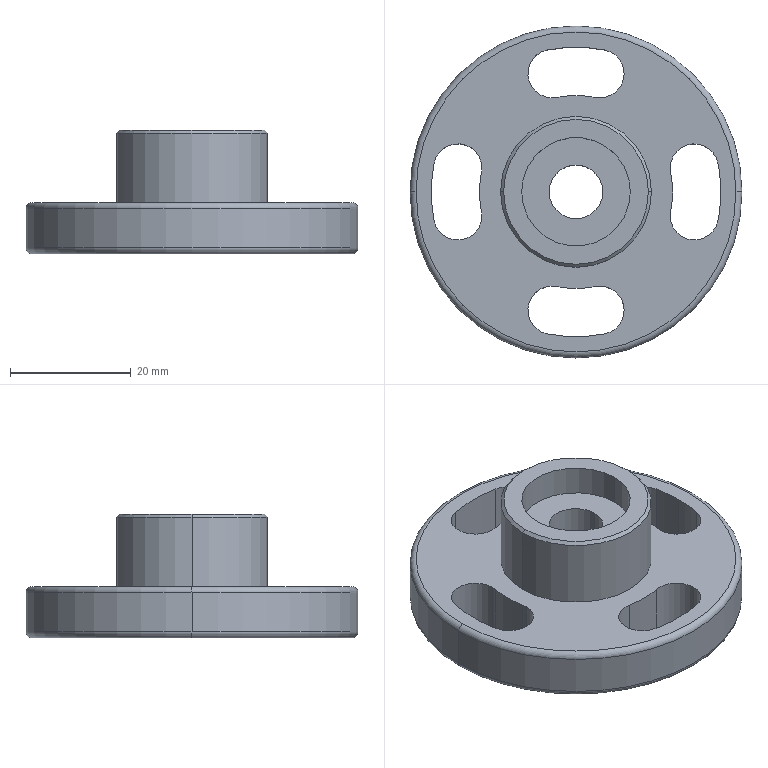Part | SolidWorks | features BaseBody 1 | 1 solid | 43 faces | box 55 x 55 x 20.5 mm | volume 18615 mm3 | cylinder 32 | plane 5 | torus 4 | cone 2 | commonest cylinder face diameters 8 x12 32 x5 48 x5 8.9 x2 15.5 x2 18 x2
STEP:
#1=CARTESIAN_POINT('',(7.973,19.601,0.));
#2=VERTEX_POINT('',#1);
#3=CARTESIAN_POINT('',(4.768,23.522,0.));
#4=VERTEX_POINT('',#3);
#5=CARTESIAN_POINT('',(3.973,19.601,0.));
#6=DIRECTION('',(0.,0.,1.));
#7=DIRECTION('',(1.,0.,0.));
#8=AXIS2_PLACEMENT_3D('',#5,#6,#7);
#9=CIRCLE('',#8,4.);
#10=EDGE_CURVE('',#2,#4,#9,.T.);
#11=ORIENTED_EDGE('',*,*,#10,.F.);
#12=CARTESIAN_POINT('',(7.973,19.601,8.5));
#13=VERTEX_POINT('',#12);
#14=CARTESIAN_POINT('',(7.973,19.601,-1.5));
#15=DIRECTION('',(0.,0.,1.));
#16=VECTOR('',#15,1000.);
#17=LINE('',#14,#16);
#18=EDGE_CURVE('',#2,#13,#17,.T.);
#19=ORIENTED_EDGE('',*,*,#18,.T.);
#20=CARTESIAN_POINT('',(4.768,23.522,8.5));
#21=VERTEX_POINT('',#20);
#22=CARTESIAN_POINT('',(3.973,19.601,8.5));
#23=DIRECTION('',(0.,0.,1.));
#24=DIRECTION('',(1.,0.,0.));
#25=AXIS2_PLACEMENT_3D('',#22,#23,#24);
#26=CIRCLE('',#25,4.);
#27=EDGE_CURVE('',#13,#21,#26,.T.);
#28=ORIENTED_EDGE('',*,*,#27,.T.);
#29=CARTESIAN_POINT('',(4.768,23.522,-1.5));
#30=DIRECTION('',(0.,0.,1.));
#31=VECTOR('',#30,1000.);
#32=LINE('',#29,#31);
#33=EDGE_CURVE('',#4,#21,#32,.T.);
#34=ORIENTED_EDGE('',*,*,#33,.F.);
#35=EDGE_LOOP('',(#11,#19,#28,#34));
#36=FACE_OUTER_BOUND('',#35,.T.);
#37=CARTESIAN_POINT('',(3.973,19.601,-1.5));
#38=DIRECTION('',(0.,0.,1.));
#39=DIRECTION('',(1.,0.,0.));
#40=AXIS2_PLACEMENT_3D('',#37,#38,#39);
#41=CYLINDRICAL_SURFACE('',#40,4.);
#42=ADVANCED_FACE('',(#36),#41,.F.);
#43=CARTESIAN_POINT('',(24.,0.,0.));
#44=VERTEX_POINT('',#43);
#45=CARTESIAN_POINT('',(23.522,4.768,0.));
#46=VERTEX_POINT('',#45);
#47=CARTESIAN_POINT('',(0.,0.,0.));
#48=DIRECTION('',(0.,0.,1.));
#49=DIRECTION('',(1.,0.,0.));
#50=AXIS2_PLACEMENT_3D('',#47,#48,#49);
#51=CIRCLE('',#50,24.);
#52=EDGE_CURVE('',#44,#46,#51,.T.);
#53=ORIENTED_EDGE('',*,*,#52,.F.);
#54=CARTESIAN_POINT('',(24.,0.,8.5));
#55=VERTEX_POINT('',#54);
#56=CARTESIAN_POINT('',(24.,0.,-1.5));
#57=DIRECTION('',(0.,0.,1.));
#58=VECTOR('',#57,1000.);
#59=LINE('',#56,#58);
#60=EDGE_CURVE('',#44,#55,#59,.T.);
#61=ORIENTED_EDGE('',*,*,#60,.T.);
#62=CARTESIAN_POINT('',(23.522,4.768,8.5));
#63=VERTEX_POINT('',#62);
#64=CARTESIAN_POINT('',(0.,0.,8.5));
#65=DIRECTION('',(0.,0.,1.));
#66=DIRECTION('',(1.,0.,0.));
#67=AXIS2_PLACEMENT_3D('',#64,#65,#66);
#68=CIRCLE('',#67,24.);
#69=EDGE_CURVE('',#55,#63,#68,.T.);
#70=ORIENTED_EDGE('',*,*,#69,.T.);
#71=CARTESIAN_POINT('',(23.522,4.768,-1.5));
#72=DIRECTION('',(0.,0.,1.));
#73=VECTOR('',#72,1000.);
#74=LINE('',#71,#73);
#75=EDGE_CURVE('',#46,#63,#74,.T.);
#76=ORIENTED_EDGE('',*,*,#75,.F.);
#77=EDGE_LOOP('',(#53,#61,#70,#76));
#78=FACE_OUTER_BOUND('',#77,.T.);
#79=CARTESIAN_POINT('',(0.,0.,-1.5));
#80=DIRECTION('',(0.,0.,1.));
#81=DIRECTION('',(1.,0.,0.));
#82=AXIS2_PLACEMENT_3D('',#79,#80,#81);
#83=CYLINDRICAL_SURFACE('',#82,24.);
#84=ADVANCED_FACE('',(#78),#83,.F.);
#85=CARTESIAN_POINT('',(16.,0.,0.));
#86=VERTEX_POINT('',#85);
#87=CARTESIAN_POINT('',(15.681,-3.179,0.));
#88=VERTEX_POINT('',#87);
#89=CARTESIAN_POINT('',(0.,0.,0.));
#90=DIRECTION('',(0.,0.,-1.));
#91=DIRECTION('',(1.,0.,0.));
#92=AXIS2_PLACEMENT_3D('',#89,#90,#91);
#93=CIRCLE('',#92,16.);
#94=EDGE_CURVE('',#86,#88,#93,.T.);
#95=ORIENTED_EDGE('',*,*,#94,.F.);
#96=CARTESIAN_POINT('',(16.,0.,8.5));
#97=VERTEX_POINT('',#96);
#98=CARTESIAN_POINT('',(16.,0.,-1.5));
#99=DIRECTION('',(0.,0.,1.));
#100=VECTOR('',#99,1000.);
#101=LINE('',#98,#100);
#102=EDGE_CURVE('',#86,#97,#101,.T.);
#103=ORIENTED_EDGE('',*,*,#102,.T.);
#104=CARTESIAN_POINT('',(15.681,-3.179,8.5));
#105=VERTEX_POINT('',#104);
#106=CARTESIAN_POINT('',(0.,0.,8.5));
#107=DIRECTION('',(0.,0.,-1.));
#108=DIRECTION('',(1.,0.,0.));
#109=AXIS2_PLACEMENT_3D('',#106,#107,#108);
#110=CIRCLE('',#109,16.);
#111=EDGE_CURVE('',#97,#105,#110,.T.);
#112=ORIENTED_EDGE('',*,*,#111,.T.);
#113=CARTESIAN_POINT('',(15.681,-3.179,-1.5));
#114=DIRECTION('',(0.,0.,1.));
#115=VECTOR('',#114,1000.);
#116=LINE('',#113,#115);
#117=EDGE_CURVE('',#88,#105,#116,.T.);
#118=ORIENTED_EDGE('',*,*,#117,.F.);
#119=EDGE_LOOP('',(#95,#103,#112,#118));
#120=FACE_OUTER_BOUND('',#119,.T.);
#121=CARTESIAN_POINT('',(0.,0.,-1.5));
#122=DIRECTION('',(0.,0.,1.));
#123=DIRECTION('',(1.,0.,0.));
#124=AXIS2_PLACEMENT_3D('',#121,#122,#123);
#125=CYLINDRICAL_SURFACE('',#124,16.);
#126=ADVANCED_FACE('',(#120),#125,.T.);
#127=CARTESIAN_POINT('',(7.973,-19.601,0.));
#128=VERTEX_POINT('',#127);
#129=CARTESIAN_POINT('',(3.179,-15.681,0.));
#130=VERTEX_POINT('',#129);
#131=CARTESIAN_POINT('',(3.973,-19.601,0.));
#132=DIRECTION('',(0.,0.,1.));
#133=DIRECTION('',(1.,0.,0.));
#134=AXIS2_PLACEMENT_3D('',#131,#132,#133);
#135=CIRCLE('',#134,4.);
#136=EDGE_CURVE('',#128,#130,#135,.T.);
#137=ORIENTED_EDGE('',*,*,#136,.F.);
#138=CARTESIAN_POINT('',(7.973,-19.601,8.5));
#139=VERTEX_POINT('',#138);
#140=CARTESIAN_POINT('',(7.973,-19.601,-1.5));
#141=DIRECTION('',(0.,0.,1.));
#142=VECTOR('',#141,1000.);
#143=LINE('',#140,#142);
#144=EDGE_CURVE('',#128,#139,#143,.T.);
#145=ORIENTED_EDGE('',*,*,#144,.T.);
#146=CARTESIAN_POINT('',(3.179,-15.681,8.5));
#147=VERTEX_POINT('',#146);
#148=CARTESIAN_POINT('',(3.973,-19.601,8.5));
#149=DIRECTION('',(0.,0.,1.));
#150=DIRECTION('',(1.,0.,0.));
#151=AXIS2_PLACEMENT_3D('',#148,#149,#150);
#152=CIRCLE('',#151,4.);
#153=EDGE_CURVE('',#139,#147,#152,.T.);
#154=ORIENTED_EDGE('',*,*,#153,.T.);
#155=CARTESIAN_POINT('',(3.179,-15.681,-1.5));
#156=DIRECTION('',(0.,0.,1.));
#157=VECTOR('',#156,1000.);
#158=LINE('',#155,#157);
#159=EDGE_CURVE('',#130,#147,#158,.T.);
#160=ORIENTED_EDGE('',*,*,#159,.F.);
#161=EDGE_LOOP('',(#137,#145,#154,#160));
#162=FACE_OUTER_BOUND('',#161,.T.);
#163=CARTESIAN_POINT('',(3.973,-19.601,-1.5));
#164=DIRECTION('',(0.,0.,1.));
#165=DIRECTION('',(1.,0.,0.));
#166=AXIS2_PLACEMENT_3D('',#163,#164,#165);
#167=CYLINDRICAL_SURFACE('',#166,4.);
#168=ADVANCED_FACE('',(#162),#167,.F.);
#169=CARTESIAN_POINT('',(-15.601,-3.973,0.));
#170=VERTEX_POINT('',#169);
#171=CARTESIAN_POINT('',(-15.681,-3.179,0.));
#172=VERTEX_POINT('',#171);
#173=CARTESIAN_POINT('',(-19.601,-3.973,0.));
#174=DIRECTION('',(0.,0.,1.));
#175=DIRECTION('',(1.,0.,0.));
#176=AXIS2_PLACEMENT_3D('',#173,#174,#175);
#177=CIRCLE('',#176,4.);
#178=EDGE_CURVE('',#170,#172,#177,.T.);
#179=ORIENTED_EDGE('',*,*,#178,.F.);
#180=CARTESIAN_POINT('',(-15.601,-3.973,8.5));
#181=VERTEX_POINT('',#180);
#182=CARTESIAN_POINT('',(-15.601,-3.973,-1.5));
#183=DIRECTION('',(0.,0.,1.));
#184=VECTOR('',#183,1000.);
#185=LINE('',#182,#184);
#186=EDGE_CURVE('',#170,#181,#185,.T.);
#187=ORIENTED_EDGE('',*,*,#186,.T.);
#188=CARTESIAN_POINT('',(-15.681,-3.179,8.5));
#189=VERTEX_POINT('',#188);
#190=CARTESIAN_POINT('',(-19.601,-3.973,8.5));
#191=DIRECTION('',(0.,0.,1.));
#192=DIRECTION('',(1.,0.,0.));
#193=AXIS2_PLACEMENT_3D('',#190,#191,#192);
#194=CIRCLE('',#193,4.);
#195=EDGE_CURVE('',#181,#189,#194,.T.);
#196=ORIENTED_EDGE('',*,*,#195,.T.);
#197=CARTESIAN_POINT('',(-15.681,-3.179,-1.5));
#198=DIRECTION('',(0.,0.,1.));
#199=VECTOR('',#198,1000.);
#200=LINE('',#197,#199);
#201=EDGE_CURVE('',#172,#189,#200,.T.);
#202=ORIENTED_EDGE('',*,*,#201,.F.);
#203=EDGE_LOOP('',(#179,#187,#196,#202));
#204=FACE_OUTER_BOUND('',#203,.T.);
#205=CARTESIAN_POINT('',(-19.601,-3.973,-1.5));
#206=DIRECTION('',(0.,0.,1.));
#207=DIRECTION('',(1.,0.,0.));
#208=AXIS2_PLACEMENT_3D('',#205,#206,#207);
#209=CYLINDRICAL_SURFACE('',#208,4.);
#210=ADVANCED_FACE('',(#204),#209,.F.);
#211=CARTESIAN_POINT('',(-15.601,3.973,0.));
#212=VERTEX_POINT('',#211);
#213=CARTESIAN_POINT('',(-23.522,4.768,0.));
#214=VERTEX_POINT('',#213);
#215=CARTESIAN_POINT('',(-19.601,3.973,0.));
#216=DIRECTION('',(0.,0.,1.));
#217=DIRECTION('',(1.,0.,0.));
#218=AXIS2_PLACEMENT_3D('',#215,#216,#217);
#219=CIRCLE('',#218,4.);
#220=EDGE_CURVE('',#212,#214,#219,.T.);
#221=ORIENTED_EDGE('',*,*,#220,.F.);
#222=CARTESIAN_POINT('',(-15.601,3.973,8.5));
#223=VERTEX_POINT('',#222);
#224=CARTESIAN_POINT('',(-15.601,3.973,-1.5));
#225=DIRECTION('',(0.,0.,1.));
#226=VECTOR('',#225,1000.);
#227=LINE('',#224,#226);
#228=EDGE_CURVE('',#212,#223,#227,.T.);
#229=ORIENTED_EDGE('',*,*,#228,.T.);
#230=CARTESIAN_POINT('',(-23.522,4.768,8.5));
#231=VERTEX_POINT('',#230);
#232=CARTESIAN_POINT('',(-19.601,3.973,8.5));
#233=DIRECTION('',(0.,0.,1.));
#234=DIRECTION('',(1.,0.,0.));
#235=AXIS2_PLACEMENT_3D('',#232,#233,#234);
#236=CIRCLE('',#235,4.);
#237=EDGE_CURVE('',#223,#231,#236,.T.);
#238=ORIENTED_EDGE('',*,*,#237,.T.);
#239=CARTESIAN_POINT('',(-23.522,4.768,-1.5));
#240=DIRECTION('',(0.,0.,1.));
#241=VECTOR('',#240,1000.);
#242=LINE('',#239,#241);
#243=EDGE_CURVE('',#214,#231,#242,.T.);
#244=ORIENTED_EDGE('',*,*,#243,.F.);
#245=EDGE_LOOP('',(#221,#229,#238,#244));
#246=FACE_OUTER_BOUND('',#245,.T.);
#247=CARTESIAN_POINT('',(-19.601,3.973,-1.5));
#248=DIRECTION('',(0.,0.,1.));
#249=DIRECTION('',(1.,0.,0.));
#250=AXIS2_PLACEMENT_3D('',#247,#248,#249);
#251=CYLINDRICAL_SURFACE('',#250,4.);
#252=ADVANCED_FACE('',(#246),#251,.F.);
#253=CARTESIAN_POINT('',(-27.5,0.,7.5));
#254=VERTEX_POINT('',#253);
#255=CARTESIAN_POINT('',(27.5,0.,7.5));
#256=VERTEX_POINT('',#255);
#257=CARTESIAN_POINT('',(0.,0.,7.5));
#258=DIRECTION('',(0.,0.,-1.));
#259=DIRECTION('',(1.,0.,0.));
#260=AXIS2_PLACEMENT_3D('',#257,#258,#259);
#261=CIRCLE('',#260,27.5);
#262=EDGE_CURVE('',#254,#256,#261,.T.);
#263=ORIENTED_EDGE('',*,*,#262,.F.);
#264=CARTESIAN_POINT('',(-26.5,0.,8.5));
#265=VERTEX_POINT('',#264);
#266=CARTESIAN_POINT('',(-26.5,0.,7.5));
#267=DIRECTION('',(0.,1.,0.));
#268=DIRECTION('',(-1.,0.,0.));
#269=AXIS2_PLACEMENT_3D('',#266,#267,#268);
#270=CIRCLE('',#269,1.);
#271=EDGE_CURVE('',#254,#265,#270,.T.);
#272=ORIENTED_EDGE('',*,*,#271,.T.);
#273=CARTESIAN_POINT('',(26.5,0.,8.5));
#274=VERTEX_POINT('',#273);
#275=CARTESIAN_POINT('',(0.,0.,8.5));
#276=DIRECTION('',(0.,0.,1.));
#277=DIRECTION('',(1.,0.,0.));
#278=AXIS2_PLACEMENT_3D('',#275,#276,#277);
#279=CIRCLE('',#278,26.5);
#280=EDGE_CURVE('',#274,#265,#279,.T.);
#281=ORIENTED_EDGE('',*,*,#280,.F.);
#282=CARTESIAN_POINT('',(26.5,0.,7.5));
#283=DIRECTION('',(0.,-1.,0.));
#284=DIRECTION('',(0.,0.,-1.));
#285=AXIS2_PLACEMENT_3D('',#282,#283,#284);
#286=CIRCLE('',#285,1.);
#287=EDGE_CURVE('',#256,#274,#286,.T.);
#288=ORIENTED_EDGE('',*,*,#287,.F.);
#289=EDGE_LOOP('',(#263,#272,#281,#288));
#290=FACE_OUTER_BOUND('',#289,.T.);
#291=CARTESIAN_POINT('',(0.,0.,7.5));
#292=DIRECTION('',(0.,0.,1.));
#293=DIRECTION('',(1.,0.,0.));
#294=AXIS2_PLACEMENT_3D('',#291,#292,#293);
#295=TOROIDAL_SURFACE('',#294,26.5,1.);
#296=ADVANCED_FACE('',(#290),#295,.T.);
#297=CARTESIAN_POINT('',(-26.5,0.,0.));
#298=VERTEX_POINT('',#297);
#299=CARTESIAN_POINT('',(26.5,0.,0.));
#300=VERTEX_POINT('',#299);
#301=CARTESIAN_POINT('',(0.,0.,0.));
#302=DIRECTION('',(0.,0.,-1.));
#303=DIRECTION('',(1.,0.,0.));
#304=AXIS2_PLACEMENT_3D('',#301,#302,#303);
#305=CIRCLE('',#304,26.5);
#306=EDGE_CURVE('',#298,#300,#305,.T.);
#307=ORIENTED_EDGE('',*,*,#306,.F.);
#308=CARTESIAN_POINT('',(-27.5,0.,1.));
#309=VERTEX_POINT('',#308);
#310=CARTESIAN_POINT('',(-26.5,0.,1.));
#311=DIRECTION('',(0.,1.,0.));
#312=DIRECTION('',(-1.,0.,0.));
#313=AXIS2_PLACEMENT_3D('',#310,#311,#312);
#314=CIRCLE('',#313,1.);
#315=EDGE_CURVE('',#298,#309,#314,.T.);
#316=ORIENTED_EDGE('',*,*,#315,.T.);
#317=CARTESIAN_POINT('',(27.5,0.,1.));
#318=VERTEX_POINT('',#317);
#319=CARTESIAN_POINT('',(0.,0.,1.));
#320=DIRECTION('',(0.,0.,1.));
#321=DIRECTION('',(1.,0.,0.));
#322=AXIS2_PLACEMENT_3D('',#319,#320,#321);
#323=CIRCLE('',#322,27.5);
#324=EDGE_CURVE('',#318,#309,#323,.T.);
#325=ORIENTED_EDGE('',*,*,#324,.F.);
#326=CARTESIAN_POINT('',(26.5,0.,1.));
#327=DIRECTION('',(0.,-1.,0.));
#328=DIRECTION('',(0.,0.,-1.));
#329=AXIS2_PLACEMENT_3D('',#326,#327,#328);
#330=CIRCLE('',#329,1.);
#331=EDGE_CURVE('',#300,#318,#330,.T.);
#332=ORIENTED_EDGE('',*,*,#331,.F.);
#333=EDGE_LOOP('',(#307,#316,#325,#332));
#334=FACE_OUTER_BOUND('',#333,.T.);
#335=CARTESIAN_POINT('',(0.,0.,1.));
#336=DIRECTION('',(0.,0.,1.));
#337=DIRECTION('',(1.,0.,0.));
#338=AXIS2_PLACEMENT_3D('',#335,#336,#337);
#339=TOROIDAL_SURFACE('',#338,26.5,1.);
#340=ADVANCED_FACE('',(#334),#339,.T.);
#341=CARTESIAN_POINT('',(12.,0.,20.5));
#342=VERTEX_POINT('',#341);
#343=CARTESIAN_POINT('',(-12.,0.,20.5));
#344=VERTEX_POINT('',#343);
#345=CARTESIAN_POINT('',(0.,0.,20.5));
#346=DIRECTION('',(0.,0.,1.));
#347=DIRECTION('',(1.,0.,0.));
#348=AXIS2_PLACEMENT_3D('',#345,#346,#347);
#349=CIRCLE('',#348,12.);
#350=EDGE_CURVE('',#342,#344,#349,.T.);
#351=ORIENTED_EDGE('',*,*,#350,.F.);
#352=CARTESIAN_POINT('',(12.5,0.,20.));
#353=VERTEX_POINT('',#352);
#354=CARTESIAN_POINT('',(12.,0.,20.5));
#355=DIRECTION('',(0.7071,0.,-0.7071));
#356=VECTOR('',#355,1000.);
#357=LINE('',#354,#356);
#358=EDGE_CURVE('',#342,#353,#357,.T.);
#359=ORIENTED_EDGE('',*,*,#358,.T.);
#360=CARTESIAN_POINT('',(-12.5,0.,20.));
#361=VERTEX_POINT('',#360);
#362=CARTESIAN_POINT('',(0.,0.,20.));
#363=DIRECTION('',(0.,0.,-1.));
#364=DIRECTION('',(1.,0.,0.));
#365=AXIS2_PLACEMENT_3D('',#362,#363,#364);
#366=CIRCLE('',#365,12.5);
#367=EDGE_CURVE('',#361,#353,#366,.T.);
#368=ORIENTED_EDGE('',*,*,#367,.F.);
#369=CARTESIAN_POINT('',(-12.,0.,20.5));
#370=DIRECTION('',(-0.7071,0.,-0.7071));
#371=VECTOR('',#370,1000.);
#372=LINE('',#369,#371);
#373=EDGE_CURVE('',#344,#361,#372,.T.);
#374=ORIENTED_EDGE('',*,*,#373,.F.);
#375=EDGE_LOOP('',(#351,#359,#368,#374));
#376=FACE_OUTER_BOUND('',#375,.T.);
#377=CARTESIAN_POINT('',(0.,0.,20.5));
#378=DIRECTION('',(0.,0.,-1.));
#379=DIRECTION('',(-1.,0.,0.));
#380=AXIS2_PLACEMENT_3D('',#377,#378,#379);
#381=CONICAL_SURFACE('',#380,12.,0.7854);
#382=ADVANCED_FACE('',(#376),#381,.T.);
#383=CARTESIAN_POINT('',(-9.,0.,15.5));
#384=VERTEX_POINT('',#383);
#385=CARTESIAN_POINT('',(9.,0.,15.5));
#386=VERTEX_POINT('',#385);
#387=CARTESIAN_POINT('',(0.,0.,15.5));
#388=DIRECTION('',(0.,0.,1.));
#389=DIRECTION('',(1.,0.,0.));
#390=AXIS2_PLACEMENT_3D('',#387,#388,#389);
#391=CIRCLE('',#390,9.);
#392=EDGE_CURVE('',#384,#386,#391,.T.);
#393=ORIENTED_EDGE('',*,*,#392,.F.);
#394=CARTESIAN_POINT('',(-9.,0.,20.5));
#395=VERTEX_POINT('',#394);
#396=CARTESIAN_POINT('',(-9.,0.,15.5));
#397=DIRECTION('',(0.,0.,1.));
#398=VECTOR('',#397,1000.);
#399=LINE('',#396,#398);
#400=EDGE_CURVE('',#384,#395,#399,.T.);
#401=ORIENTED_EDGE('',*,*,#400,.T.);
#402=CARTESIAN_POINT('',(9.,0.,20.5));
#403=VERTEX_POINT('',#402);
#404=CARTESIAN_POINT('',(0.,0.,20.5));
#405=DIRECTION('',(0.,0.,1.));
#406=DIRECTION('',(1.,0.,0.));
#407=AXIS2_PLACEMENT_3D('',#404,#405,#406);
#408=CIRCLE('',#407,9.);
#409=EDGE_CURVE('',#395,#403,#408,.T.);
#410=ORIENTED_EDGE('',*,*,#409,.T.);
#411=CARTESIAN_POINT('',(9.,0.,15.5));
#412=DIRECTION('',(0.,0.,1.));
#413=VECTOR('',#412,1000.);
#414=LINE('',#411,#413);
#415=EDGE_CURVE('',#386,#403,#414,.T.);
#416=ORIENTED_EDGE('',*,*,#415,.F.);
#417=EDGE_LOOP('',(#393,#401,#410,#416));
#418=FACE_OUTER_BOUND('',#417,.T.);
#419=CARTESIAN_POINT('',(0.,0.,15.5));
#420=DIRECTION('',(0.,0.,1.));
#421=DIRECTION('',(1.,0.,0.));
#422=AXIS2_PLACEMENT_3D('',#419,#420,#421);
#423=CYLINDRICAL_SURFACE('',#422,9.);
#424=ADVANCED_FACE('',(#418),#423,.F.);
#425=CARTESIAN_POINT('',(7.75,0.,10.));
#426=VERTEX_POINT('',#425);
#427=CARTESIAN_POINT('',(-7.75,0.,10.));
#428=VERTEX_POINT('',#427);
#429=CARTESIAN_POINT('',(0.,0.,10.));
#430=DIRECTION('',(0.,0.,-1.));
#431=DIRECTION('',(-1.,0.,0.));
#432=AXIS2_PLACEMENT_3D('',#429,#430,#431);
#433=CIRCLE('',#432,7.75);
#434=EDGE_CURVE('',#426,#428,#433,.T.);
#435=ORIENTED_EDGE('',*,*,#434,.F.);
#436=CARTESIAN_POINT('',(7.75,0.,0.));
#437=VERTEX_POINT('',#436);
#438=CARTESIAN_POINT('',(7.75,0.,10.));
#439=DIRECTION('',(0.,0.,-1.));
#440=VECTOR('',#439,1000.);
#441=LINE('',#438,#440);
#442=EDGE_CURVE('',#426,#437,#441,.T.);
#443=ORIENTED_EDGE('',*,*,#442,.T.);
#444=CARTESIAN_POINT('',(-7.75,0.,0.));
#445=VERTEX_POINT('',#444);
#446=CARTESIAN_POINT('',(0.,0.,0.));
#447=DIRECTION('',(0.,0.,-1.));
#448=DIRECTION('',(-1.,0.,0.));
#449=AXIS2_PLACEMENT_3D('',#446,#447,#448);
#450=CIRCLE('',#449,7.75);
#451=EDGE_CURVE('',#437,#445,#450,.T.);
#452=ORIENTED_EDGE('',*,*,#451,.T.);
#453=CARTESIAN_POINT('',(-7.75,0.,10.));
#454=DIRECTION('',(0.,0.,-1.));
#455=VECTOR('',#454,1000.);
#456=LINE('',#453,#455);
#457=EDGE_CURVE('',#428,#445,#456,.T.);
#458=ORIENTED_EDGE('',*,*,#457,.F.);
#459=EDGE_LOOP('',(#435,#443,#452,#458));
#460=FACE_OUTER_BOUND('',#459,.T.);
#461=CARTESIAN_POINT('',(0.,0.,10.));
#462=DIRECTION('',(0.,0.,-1.));
#463=DIRECTION('',(-1.,0.,0.));
#464=AXIS2_PLACEMENT_3D('',#461,#462,#463);
#465=CYLINDRICAL_SURFACE('',#464,7.75);
#466=ADVANCED_FACE('',(#460),#465,.F.);
#467=ORIENTED_EDGE('',*,*,#367,.T.);
#468=CARTESIAN_POINT('',(12.5,0.,8.5));
#469=VERTEX_POINT('',#468);
#470=CARTESIAN_POINT('',(12.5,0.,20.5));
#471=DIRECTION('',(0.,0.,-1.));
#472=VECTOR('',#471,1000.);
#473=LINE('',#470,#472);
#474=EDGE_CURVE('',#353,#469,#473,.T.);
#475=ORIENTED_EDGE('',*,*,#474,.T.);
#476=CARTESIAN_POINT('',(-12.5,0.,8.5));
#477=VERTEX_POINT('',#476);
#478=CARTESIAN_POINT('',(0.,0.,8.5));
#479=DIRECTION('',(0.,0.,1.));
#480=DIRECTION('',(1.,0.,0.));
#481=AXIS2_PLACEMENT_3D('',#478,#479,#480);
#482=CIRCLE('',#481,12.5);
#483=EDGE_CURVE('',#469,#477,#482,.T.);
#484=ORIENTED_EDGE('',*,*,#483,.T.);
#485=CARTESIAN_POINT('',(-12.5,0.,20.5));
#486=DIRECTION('',(0.,0.,-1.));
#487=VECTOR('',#486,1000.);
#488=LINE('',#485,#487);
#489=EDGE_CURVE('',#361,#477,#488,.T.);
#490=ORIENTED_EDGE('',*,*,#489,.F.);
#491=EDGE_LOOP('',(#467,#475,#484,#490));
#492=FACE_OUTER_BOUND('',#491,.T.);
#493=CARTESIAN_POINT('',(0.,0.,20.5));
#494=DIRECTION('',(0.,0.,-1.));
#495=DIRECTION('',(-1.,0.,0.));
#496=AXIS2_PLACEMENT_3D('',#493,#494,#495);
#497=CYLINDRICAL_SURFACE('',#496,12.5);
#498=ADVANCED_FACE('',(#492),#497,.T.);
#499=ORIENTED_EDGE('',*,*,#262,.T.);
#500=CARTESIAN_POINT('',(27.5,0.,8.5));
#501=DIRECTION('',(0.,0.,-1.));
#502=VECTOR('',#501,1000.);
#503=LINE('',#500,#502);
#504=EDGE_CURVE('',#256,#318,#503,.T.);
#505=ORIENTED_EDGE('',*,*,#504,.T.);
#506=ORIENTED_EDGE('',*,*,#324,.T.);
#507=CARTESIAN_POINT('',(-27.5,0.,8.5));
#508=DIRECTION('',(0.,0.,-1.));
#509=VECTOR('',#508,1000.);
#510=LINE('',#507,#509);
#511=EDGE_CURVE('',#254,#309,#510,.T.);
#512=ORIENTED_EDGE('',*,*,#511,.F.);
#513=EDGE_LOOP('',(#499,#505,#506,#512));
#514=FACE_OUTER_BOUND('',#513,.T.);
#515=CARTESIAN_POINT('',(0.,0.,8.5));
#516=DIRECTION('',(0.,0.,-1.));
#517=DIRECTION('',(-1.,0.,0.));
#518=AXIS2_PLACEMENT_3D('',#515,#516,#517);
#519=CYLINDRICAL_SURFACE('',#518,27.5);
#520=ADVANCED_FACE('',(#514),#519,.T.);
#521=CARTESIAN_POINT('',(-4.45,0.,15.5));
#522=VERTEX_POINT('',#521);
#523=CARTESIAN_POINT('',(4.45,0.,15.5));
#524=VERTEX_POINT('',#523);
#525=CARTESIAN_POINT('',(0.,0.,15.5));
#526=DIRECTION('',(0.,0.,1.));
#527=DIRECTION('',(1.,0.,0.));
#528=AXIS2_PLACEMENT_3D('',#525,#526,#527);
#529=CIRCLE('',#528,4.45);
#530=EDGE_CURVE('',#522,#524,#529,.T.);
#531=ORIENTED_EDGE('',*,*,#530,.T.);
#532=CARTESIAN_POINT('',(4.45,0.,10.));
#533=VERTEX_POINT('',#532);
#534=CARTESIAN_POINT('',(4.45,0.,8.5));
#535=DIRECTION('',(0.,0.,-1.));
#536=VECTOR('',#535,1000.);
#537=LINE('',#534,#536);
#538=EDGE_CURVE('',#524,#533,#537,.T.);
#539=ORIENTED_EDGE('',*,*,#538,.T.);
#540=CARTESIAN_POINT('',(-4.45,0.,10.));
#541=VERTEX_POINT('',#540);
#542=CARTESIAN_POINT('',(0.,0.,10.));
#543=DIRECTION('',(0.,0.,-1.));
#544=DIRECTION('',(-1.,0.,0.));
#545=AXIS2_PLACEMENT_3D('',#542,#543,#544);
#546=CIRCLE('',#545,4.45);
#547=EDGE_CURVE('',#533,#541,#546,.T.);
#548=ORIENTED_EDGE('',*,*,#547,.T.);
#549=CARTESIAN_POINT('',(-4.45,0.,8.5));
#550=DIRECTION('',(0.,0.,-1.));
#551=VECTOR('',#550,1000.);
#552=LINE('',#549,#551);
#553=EDGE_CURVE('',#522,#541,#552,.T.);
#554=ORIENTED_EDGE('',*,*,#553,.F.);
#555=EDGE_LOOP('',(#531,#539,#548,#554));
#556=FACE_OUTER_BOUND('',#555,.T.);
#557=CARTESIAN_POINT('',(0.,0.,8.5));
#558=DIRECTION('',(0.,0.,-1.));
#559=DIRECTION('',(-1.,0.,0.));
#560=AXIS2_PLACEMENT_3D('',#557,#558,#559);
#561=CYLINDRICAL_SURFACE('',#560,4.45);
#562=ADVANCED_FACE('',(#556),#561,.F.);
#563=ORIENTED_EDGE('',*,*,#538,.F.);
#564=CARTESIAN_POINT('',(0.,0.,15.5));
#565=DIRECTION('',(0.,0.,1.));
#566=DIRECTION('',(1.,0.,0.));
#567=AXIS2_PLACEMENT_3D('',#564,#565,#566);
#568=CIRCLE('',#567,4.45);
#569=EDGE_CURVE('',#524,#522,#568,.T.);
#570=ORIENTED_EDGE('',*,*,#569,.T.);
#571=ORIENTED_EDGE('',*,*,#553,.T.);
#572=CARTESIAN_POINT('',(0.,0.,10.));
#573=DIRECTION('',(0.,0.,-1.));
#574=DIRECTION('',(-1.,0.,0.));
#575=AXIS2_PLACEMENT_3D('',#572,#573,#574);
#576=CIRCLE('',#575,4.45);
#577=EDGE_CURVE('',#541,#533,#576,.T.);
#578=ORIENTED_EDGE('',*,*,#577,.T.);
#579=EDGE_LOOP('',(#563,#570,#571,#578));
#580=FACE_OUTER_BOUND('',#579,.T.);
#581=CARTESIAN_POINT('',(0.,0.,8.5));
#582=DIRECTION('',(0.,0.,-1.));
#583=DIRECTION('',(-1.,0.,0.));
#584=AXIS2_PLACEMENT_3D('',#581,#582,#583);
#585=CYLINDRICAL_SURFACE('',#584,4.45);
#586=ADVANCED_FACE('',(#580),#585,.F.);
#587=CARTESIAN_POINT('',(3.179,15.681,8.5));
#588=VERTEX_POINT('',#587);
#589=CARTESIAN_POINT('',(3.973,19.601,8.5));
#590=DIRECTION('',(0.,0.,1.));
#591=DIRECTION('',(1.,0.,0.));
#592=AXIS2_PLACEMENT_3D('',#589,#590,#591);
#593=CIRCLE('',#592,4.);
#594=EDGE_CURVE('',#588,#13,#593,.T.);
#595=ORIENTED_EDGE('',*,*,#594,.F.);
#596=CARTESIAN_POINT('',(-3.179,15.681,8.5));
#597=VERTEX_POINT('',#596);
#598=CARTESIAN_POINT('',(0.,0.,8.5));
#599=DIRECTION('',(0.,0.,-1.));
#600=DIRECTION('',(1.,0.,0.));
#601=AXIS2_PLACEMENT_3D('',#598,#599,#600);
#602=CIRCLE('',#601,16.);
#603=EDGE_CURVE('',#597,#588,#602,.T.);
#604=ORIENTED_EDGE('',*,*,#603,.F.);
#605=CARTESIAN_POINT('',(-4.768,23.522,8.5));
#606=VERTEX_POINT('',#605);
#607=CARTESIAN_POINT('',(-3.973,19.601,8.5));
#608=DIRECTION('',(0.,0.,1.));
#609=DIRECTION('',(1.,0.,0.));
#610=AXIS2_PLACEMENT_3D('',#607,#608,#609);
#611=CIRCLE('',#610,4.);
#612=EDGE_CURVE('',#606,#597,#611,.T.);
#613=ORIENTED_EDGE('',*,*,#612,.F.);
#614=CARTESIAN_POINT('',(0.,0.,8.5));
#615=DIRECTION('',(0.,0.,1.));
#616=DIRECTION('',(1.,0.,0.));
#617=AXIS2_PLACEMENT_3D('',#614,#615,#616);
#618=CIRCLE('',#617,24.);
#619=EDGE_CURVE('',#21,#606,#618,.T.);
#620=ORIENTED_EDGE('',*,*,#619,.F.);
#621=ORIENTED_EDGE('',*,*,#27,.F.);
#622=EDGE_LOOP('',(#595,#604,#613,#620,#621));
#623=FACE_BOUND('',#622,.T.);
#624=CARTESIAN_POINT('',(23.522,-4.768,8.5));
#625=VERTEX_POINT('',#624);
#626=CARTESIAN_POINT('',(19.601,-3.973,8.5));
#627=DIRECTION('',(0.,0.,1.));
#628=DIRECTION('',(1.,0.,0.));
#629=AXIS2_PLACEMENT_3D('',#626,#627,#628);
#630=CIRCLE('',#629,4.);
#631=EDGE_CURVE('',#105,#625,#630,.T.);
#632=ORIENTED_EDGE('',*,*,#631,.F.);
#633=ORIENTED_EDGE('',*,*,#111,.F.);
#634=CARTESIAN_POINT('',(15.681,3.179,8.5));
#635=VERTEX_POINT('',#634);
#636=CARTESIAN_POINT('',(0.,0.,8.5));
#637=DIRECTION('',(0.,0.,-1.));
#638=DIRECTION('',(1.,0.,0.));
#639=AXIS2_PLACEMENT_3D('',#636,#637,#638);
#640=CIRCLE('',#639,16.);
#641=EDGE_CURVE('',#635,#97,#640,.T.);
#642=ORIENTED_EDGE('',*,*,#641,.F.);
#643=CARTESIAN_POINT('',(19.601,3.973,8.5));
#644=DIRECTION('',(0.,0.,1.));
#645=DIRECTION('',(1.,0.,0.));
#646=AXIS2_PLACEMENT_3D('',#643,#644,#645);
#647=CIRCLE('',#646,4.);
#648=EDGE_CURVE('',#63,#635,#647,.T.);
#649=ORIENTED_EDGE('',*,*,#648,.F.);
#650=ORIENTED_EDGE('',*,*,#69,.F.);
#651=CARTESIAN_POINT('',(0.,0.,8.5));
#652=DIRECTION('',(0.,0.,1.));
#653=DIRECTION('',(1.,0.,0.));
#654=AXIS2_PLACEMENT_3D('',#651,#652,#653);
#655=CIRCLE('',#654,24.);
#656=EDGE_CURVE('',#625,#55,#655,.T.);
#657=ORIENTED_EDGE('',*,*,#656,.F.);
#658=EDGE_LOOP('',(#632,#633,#642,#649,#650,#657));
#659=FACE_BOUND('',#658,.T.);
#660=CARTESIAN_POINT('',(-3.179,-15.681,8.5));
#661=VERTEX_POINT('',#660);
#662=CARTESIAN_POINT('',(-4.768,-23.522,8.5));
#663=VERTEX_POINT('',#662);
#664=CARTESIAN_POINT('',(-3.973,-19.601,8.5));
#665=DIRECTION('',(0.,0.,1.));
#666=DIRECTION('',(1.,0.,0.));
#667=AXIS2_PLACEMENT_3D('',#664,#665,#666);
#668=CIRCLE('',#667,4.);
#669=EDGE_CURVE('',#661,#663,#668,.T.);
#670=ORIENTED_EDGE('',*,*,#669,.F.);
#671=CARTESIAN_POINT('',(0.,0.,8.5));
#672=DIRECTION('',(0.,0.,-1.));
#673=DIRECTION('',(1.,0.,0.));
#674=AXIS2_PLACEMENT_3D('',#671,#672,#673);
#675=CIRCLE('',#674,16.);
#676=EDGE_CURVE('',#147,#661,#675,.T.);
#677=ORIENTED_EDGE('',*,*,#676,.F.);
#678=ORIENTED_EDGE('',*,*,#153,.F.);
#679=CARTESIAN_POINT('',(4.768,-23.522,8.5));
#680=VERTEX_POINT('',#679);
#681=CARTESIAN_POINT('',(3.973,-19.601,8.5));
#682=DIRECTION('',(0.,0.,1.));
#683=DIRECTION('',(1.,0.,0.));
#684=AXIS2_PLACEMENT_3D('',#681,#682,#683);
#685=CIRCLE('',#684,4.);
#686=EDGE_CURVE('',#680,#139,#685,.T.);
#687=ORIENTED_EDGE('',*,*,#686,.F.);
#688=CARTESIAN_POINT('',(0.,0.,8.5));
#689=DIRECTION('',(0.,0.,1.));
#690=DIRECTION('',(1.,0.,0.));
#691=AXIS2_PLACEMENT_3D('',#688,#689,#690);
#692=CIRCLE('',#691,24.);
#693=EDGE_CURVE('',#663,#680,#692,.T.);
#694=ORIENTED_EDGE('',*,*,#693,.F.);
#695=EDGE_LOOP('',(#670,#677,#678,#687,#694));
#696=FACE_BOUND('',#695,.T.);
#697=CARTESIAN_POINT('',(-15.681,3.179,8.5));
#698=VERTEX_POINT('',#697);
#699=CARTESIAN_POINT('',(-19.601,3.973,8.5));
#700=DIRECTION('',(0.,0.,1.));
#701=DIRECTION('',(1.,0.,0.));
#702=AXIS2_PLACEMENT_3D('',#699,#700,#701);
#703=CIRCLE('',#702,4.);
#704=EDGE_CURVE('',#698,#223,#703,.T.);
#705=ORIENTED_EDGE('',*,*,#704,.F.);
#706=CARTESIAN_POINT('',(0.,0.,8.5));
#707=DIRECTION('',(0.,0.,-1.));
#708=DIRECTION('',(1.,0.,0.));
#709=AXIS2_PLACEMENT_3D('',#706,#707,#708);
#710=CIRCLE('',#709,16.);
#711=EDGE_CURVE('',#189,#698,#710,.T.);
#712=ORIENTED_EDGE('',*,*,#711,.F.);
#713=ORIENTED_EDGE('',*,*,#195,.F.);
#714=CARTESIAN_POINT('',(-23.522,-4.768,8.5));
#715=VERTEX_POINT('',#714);
#716=CARTESIAN_POINT('',(-19.601,-3.973,8.5));
#717=DIRECTION('',(0.,0.,1.));
#718=DIRECTION('',(1.,0.,0.));
#719=AXIS2_PLACEMENT_3D('',#716,#717,#718);
#720=CIRCLE('',#719,4.);
#721=EDGE_CURVE('',#715,#181,#720,.T.);
#722=ORIENTED_EDGE('',*,*,#721,.F.);
#723=CARTESIAN_POINT('',(0.,0.,8.5));
#724=DIRECTION('',(0.,0.,1.));
#725=DIRECTION('',(1.,0.,0.));
#726=AXIS2_PLACEMENT_3D('',#723,#724,#725);
#727=CIRCLE('',#726,24.);
#728=EDGE_CURVE('',#231,#715,#727,.T.);
#729=ORIENTED_EDGE('',*,*,#728,.F.);
#730=ORIENTED_EDGE('',*,*,#237,.F.);
#731=EDGE_LOOP('',(#705,#712,#713,#722,#729,#730));
#732=FACE_BOUND('',#731,.T.);
#733=ORIENTED_EDGE('',*,*,#280,.T.);
#734=CARTESIAN_POINT('',(0.,0.,8.5));
#735=DIRECTION('',(0.,0.,1.));
#736=DIRECTION('',(1.,0.,0.));
#737=AXIS2_PLACEMENT_3D('',#734,#735,#736);
#738=CIRCLE('',#737,26.5);
#739=EDGE_CURVE('',#265,#274,#738,.T.);
#740=ORIENTED_EDGE('',*,*,#739,.T.);
#741=EDGE_LOOP('',(#733,#740));
#742=FACE_OUTER_BOUND('',#741,.T.);
#743=CARTESIAN_POINT('',(0.,0.,8.5));
#744=DIRECTION('',(0.,0.,1.));
#745=DIRECTION('',(1.,0.,0.));
#746=AXIS2_PLACEMENT_3D('',#743,#744,#745);
#747=CIRCLE('',#746,12.5);
#748=EDGE_CURVE('',#477,#469,#747,.T.);
#749=ORIENTED_EDGE('',*,*,#748,.F.);
#750=ORIENTED_EDGE('',*,*,#483,.F.);
#751=EDGE_LOOP('',(#749,#750));
#752=FACE_BOUND('',#751,.T.);
#753=CARTESIAN_POINT('',(0.,0.,8.5));
#754=DIRECTION('',(0.,0.,1.));
#755=DIRECTION('',(1.,0.,0.));
#756=AXIS2_PLACEMENT_3D('',#753,#754,#755);
#757=PLANE('',#756);
#758=ADVANCED_FACE('',(#623,#659,#696,#732,#742,#752),#757,.T.);
#759=CARTESIAN_POINT('',(-3.179,15.681,0.));
#760=VERTEX_POINT('',#759);
#761=CARTESIAN_POINT('',(3.179,15.681,0.));
#762=VERTEX_POINT('',#761);
#763=CARTESIAN_POINT('',(0.,0.,0.));
#764=DIRECTION('',(0.,0.,-1.));
#765=DIRECTION('',(1.,0.,0.));
#766=AXIS2_PLACEMENT_3D('',#763,#764,#765);
#767=CIRCLE('',#766,16.);
#768=EDGE_CURVE('',#760,#762,#767,.T.);
#769=ORIENTED_EDGE('',*,*,#768,.T.);
#770=CARTESIAN_POINT('',(3.973,19.601,0.));
#771=DIRECTION('',(0.,0.,1.));
#772=DIRECTION('',(1.,0.,0.));
#773=AXIS2_PLACEMENT_3D('',#770,#771,#772);
#774=CIRCLE('',#773,4.);
#775=EDGE_CURVE('',#762,#2,#774,.T.);
#776=ORIENTED_EDGE('',*,*,#775,.T.);
#777=ORIENTED_EDGE('',*,*,#10,.T.);
#778=CARTESIAN_POINT('',(-4.768,23.522,0.));
#779=VERTEX_POINT('',#778);
#780=CARTESIAN_POINT('',(0.,0.,0.));
#781=DIRECTION('',(0.,0.,1.));
#782=DIRECTION('',(1.,0.,0.));
#783=AXIS2_PLACEMENT_3D('',#780,#781,#782);
#784=CIRCLE('',#783,24.);
#785=EDGE_CURVE('',#4,#779,#784,.T.);
#786=ORIENTED_EDGE('',*,*,#785,.T.);
#787=CARTESIAN_POINT('',(-3.973,19.601,0.));
#788=DIRECTION('',(0.,0.,1.));
#789=DIRECTION('',(1.,0.,0.));
#790=AXIS2_PLACEMENT_3D('',#787,#788,#789);
#791=CIRCLE('',#790,4.);
#792=EDGE_CURVE('',#779,#760,#791,.T.);
#793=ORIENTED_EDGE('',*,*,#792,.T.);
#794=EDGE_LOOP('',(#769,#776,#777,#786,#793));
#795=FACE_BOUND('',#794,.T.);
#796=CARTESIAN_POINT('',(15.681,3.179,0.));
#797=VERTEX_POINT('',#796);
#798=CARTESIAN_POINT('',(0.,0.,0.));
#799=DIRECTION('',(0.,0.,-1.));
#800=DIRECTION('',(1.,0.,0.));
#801=AXIS2_PLACEMENT_3D('',#798,#799,#800);
#802=CIRCLE('',#801,16.);
#803=EDGE_CURVE('',#797,#86,#802,.T.);
#804=ORIENTED_EDGE('',*,*,#803,.T.);
#805=ORIENTED_EDGE('',*,*,#94,.T.);
#806=CARTESIAN_POINT('',(23.522,-4.768,0.));
#807=VERTEX_POINT('',#806);
#808=CARTESIAN_POINT('',(19.601,-3.973,0.));
#809=DIRECTION('',(0.,0.,1.));
#810=DIRECTION('',(1.,0.,0.));
#811=AXIS2_PLACEMENT_3D('',#808,#809,#810);
#812=CIRCLE('',#811,4.);
#813=EDGE_CURVE('',#88,#807,#812,.T.);
#814=ORIENTED_EDGE('',*,*,#813,.T.);
#815=CARTESIAN_POINT('',(0.,0.,0.));
#816=DIRECTION('',(0.,0.,1.));
#817=DIRECTION('',(1.,0.,0.));
#818=AXIS2_PLACEMENT_3D('',#815,#816,#817);
#819=CIRCLE('',#818,24.);
#820=EDGE_CURVE('',#807,#44,#819,.T.);
#821=ORIENTED_EDGE('',*,*,#820,.T.);
#822=ORIENTED_EDGE('',*,*,#52,.T.);
#823=CARTESIAN_POINT('',(19.601,3.973,0.));
#824=DIRECTION('',(0.,0.,1.));
#825=DIRECTION('',(1.,0.,0.));
#826=AXIS2_PLACEMENT_3D('',#823,#824,#825);
#827=CIRCLE('',#826,4.);
#828=EDGE_CURVE('',#46,#797,#827,.T.);
#829=ORIENTED_EDGE('',*,*,#828,.T.);
#830=EDGE_LOOP('',(#804,#805,#814,#821,#822,#829));
#831=FACE_BOUND('',#830,.T.);
#832=CARTESIAN_POINT('',(-3.179,-15.681,0.));
#833=VERTEX_POINT('',#832);
#834=CARTESIAN_POINT('',(0.,0.,0.));
#835=DIRECTION('',(0.,0.,-1.));
#836=DIRECTION('',(1.,0.,0.));
#837=AXIS2_PLACEMENT_3D('',#834,#835,#836);
#838=CIRCLE('',#837,16.);
#839=EDGE_CURVE('',#130,#833,#838,.T.);
#840=ORIENTED_EDGE('',*,*,#839,.T.);
#841=CARTESIAN_POINT('',(-4.768,-23.522,0.));
#842=VERTEX_POINT('',#841);
#843=CARTESIAN_POINT('',(-3.973,-19.601,0.));
#844=DIRECTION('',(0.,0.,1.));
#845=DIRECTION('',(1.,0.,0.));
#846=AXIS2_PLACEMENT_3D('',#843,#844,#845);
#847=CIRCLE('',#846,4.);
#848=EDGE_CURVE('',#833,#842,#847,.T.);
#849=ORIENTED_EDGE('',*,*,#848,.T.);
#850=CARTESIAN_POINT('',(4.768,-23.522,0.));
#851=VERTEX_POINT('',#850);
#852=CARTESIAN_POINT('',(0.,0.,0.));
#853=DIRECTION('',(0.,0.,1.));
#854=DIRECTION('',(1.,0.,0.));
#855=AXIS2_PLACEMENT_3D('',#852,#853,#854);
#856=CIRCLE('',#855,24.);
#857=EDGE_CURVE('',#842,#851,#856,.T.);
#858=ORIENTED_EDGE('',*,*,#857,.T.);
#859=CARTESIAN_POINT('',(3.973,-19.601,0.));
#860=DIRECTION('',(0.,0.,1.));
#861=DIRECTION('',(1.,0.,0.));
#862=AXIS2_PLACEMENT_3D('',#859,#860,#861);
#863=CIRCLE('',#862,4.);
#864=EDGE_CURVE('',#851,#128,#863,.T.);
#865=ORIENTED_EDGE('',*,*,#864,.T.);
#866=ORIENTED_EDGE('',*,*,#136,.T.);
#867=EDGE_LOOP('',(#840,#849,#858,#865,#866));
#868=FACE_BOUND('',#867,.T.);
#869=CARTESIAN_POINT('',(-15.681,3.179,0.));
#870=VERTEX_POINT('',#869);
#871=CARTESIAN_POINT('',(0.,0.,0.));
#872=DIRECTION('',(0.,0.,-1.));
#873=DIRECTION('',(1.,0.,0.));
#874=AXIS2_PLACEMENT_3D('',#871,#872,#873);
#875=CIRCLE('',#874,16.);
#876=EDGE_CURVE('',#172,#870,#875,.T.);
#877=ORIENTED_EDGE('',*,*,#876,.T.);
#878=CARTESIAN_POINT('',(-19.601,3.973,0.));
#879=DIRECTION('',(0.,0.,1.));
#880=DIRECTION('',(1.,0.,0.));
#881=AXIS2_PLACEMENT_3D('',#878,#879,#880);
#882=CIRCLE('',#881,4.);
#883=EDGE_CURVE('',#870,#212,#882,.T.);
#884=ORIENTED_EDGE('',*,*,#883,.T.);
#885=ORIENTED_EDGE('',*,*,#220,.T.);
#886=CARTESIAN_POINT('',(-23.522,-4.768,0.));
#887=VERTEX_POINT('',#886);
#888=CARTESIAN_POINT('',(0.,0.,0.));
#889=DIRECTION('',(0.,0.,1.));
#890=DIRECTION('',(1.,0.,0.));
#891=AXIS2_PLACEMENT_3D('',#888,#889,#890);
#892=CIRCLE('',#891,24.);
#893=EDGE_CURVE('',#214,#887,#892,.T.);
#894=ORIENTED_EDGE('',*,*,#893,.T.);
#895=CARTESIAN_POINT('',(-19.601,-3.973,0.));
#896=DIRECTION('',(0.,0.,1.));
#897=DIRECTION('',(1.,0.,0.));
#898=AXIS2_PLACEMENT_3D('',#895,#896,#897);
#899=CIRCLE('',#898,4.);
#900=EDGE_CURVE('',#887,#170,#899,.T.);
#901=ORIENTED_EDGE('',*,*,#900,.T.);
#902=ORIENTED_EDGE('',*,*,#178,.T.);
#903=EDGE_LOOP('',(#877,#884,#885,#894,#901,#902));
#904=FACE_BOUND('',#903,.T.);
#905=CARTESIAN_POINT('',(0.,0.,0.));
#906=DIRECTION('',(0.,0.,-1.));
#907=DIRECTION('',(1.,0.,0.));
#908=AXIS2_PLACEMENT_3D('',#905,#906,#907);
#909=CIRCLE('',#908,26.5);
#910=EDGE_CURVE('',#300,#298,#909,.T.);
#911=ORIENTED_EDGE('',*,*,#910,.T.);
#912=ORIENTED_EDGE('',*,*,#306,.T.);
#913=EDGE_LOOP('',(#911,#912));
#914=FACE_OUTER_BOUND('',#913,.T.);
#915=CARTESIAN_POINT('',(0.,0.,0.));
#916=DIRECTION('',(0.,0.,-1.));
#917=DIRECTION('',(-1.,0.,0.));
#918=AXIS2_PLACEMENT_3D('',#915,#916,#917);
#919=CIRCLE('',#918,7.75);
#920=EDGE_CURVE('',#445,#437,#919,.T.);
#921=ORIENTED_EDGE('',*,*,#920,.F.);
#922=ORIENTED_EDGE('',*,*,#451,.F.);
#923=EDGE_LOOP('',(#921,#922));
#924=FACE_BOUND('',#923,.T.);
#925=CARTESIAN_POINT('',(0.,0.,0.));
#926=DIRECTION('',(0.,0.,1.));
#927=DIRECTION('',(1.,0.,0.));
#928=AXIS2_PLACEMENT_3D('',#925,#926,#927);
#929=PLANE('',#928);
#930=ADVANCED_FACE('',(#795,#831,#868,#904,#914,#924),#929,.F.);
#931=ORIENTED_EDGE('',*,*,#504,.F.);
#932=CARTESIAN_POINT('',(0.,0.,7.5));
#933=DIRECTION('',(0.,0.,-1.));
#934=DIRECTION('',(1.,0.,0.));
#935=AXIS2_PLACEMENT_3D('',#932,#933,#934);
#936=CIRCLE('',#935,27.5);
#937=EDGE_CURVE('',#256,#254,#936,.T.);
#938=ORIENTED_EDGE('',*,*,#937,.T.);
#939=ORIENTED_EDGE('',*,*,#511,.T.);
#940=CARTESIAN_POINT('',(0.,0.,1.));
#941=DIRECTION('',(0.,0.,1.));
#942=DIRECTION('',(1.,0.,0.));
#943=AXIS2_PLACEMENT_3D('',#940,#941,#942);
#944=CIRCLE('',#943,27.5);
#945=EDGE_CURVE('',#309,#318,#944,.T.);
#946=ORIENTED_EDGE('',*,*,#945,.T.);
#947=EDGE_LOOP('',(#931,#938,#939,#946));
#948=FACE_OUTER_BOUND('',#947,.T.);
#949=CARTESIAN_POINT('',(0.,0.,8.5));
#950=DIRECTION('',(0.,0.,-1.));
#951=DIRECTION('',(-1.,0.,0.));
#952=AXIS2_PLACEMENT_3D('',#949,#950,#951);
#953=CYLINDRICAL_SURFACE('',#952,27.5);
#954=ADVANCED_FACE('',(#948),#953,.T.);
#955=CARTESIAN_POINT('',(0.,0.,20.5));
#956=DIRECTION('',(0.,0.,1.));
#957=DIRECTION('',(1.,0.,0.));
#958=AXIS2_PLACEMENT_3D('',#955,#956,#957);
#959=CIRCLE('',#958,12.);
#960=EDGE_CURVE('',#344,#342,#959,.T.);
#961=ORIENTED_EDGE('',*,*,#960,.T.);
#962=ORIENTED_EDGE('',*,*,#350,.T.);
#963=EDGE_LOOP('',(#961,#962));
#964=FACE_OUTER_BOUND('',#963,.T.);
#965=CARTESIAN_POINT('',(0.,0.,20.5));
#966=DIRECTION('',(0.,0.,1.));
#967=DIRECTION('',(1.,0.,0.));
#968=AXIS2_PLACEMENT_3D('',#965,#966,#967);
#969=CIRCLE('',#968,9.);
#970=EDGE_CURVE('',#403,#395,#969,.T.);
#971=ORIENTED_EDGE('',*,*,#970,.F.);
#972=ORIENTED_EDGE('',*,*,#409,.F.);
#973=EDGE_LOOP('',(#971,#972));
#974=FACE_BOUND('',#973,.T.);
#975=CARTESIAN_POINT('',(0.,0.,20.5));
#976=DIRECTION('',(0.,0.,1.));
#977=DIRECTION('',(1.,0.,0.));
#978=AXIS2_PLACEMENT_3D('',#975,#976,#977);
#979=PLANE('',#978);
#980=ADVANCED_FACE('',(#964,#974),#979,.T.);
#981=ORIENTED_EDGE('',*,*,#474,.F.);
#982=CARTESIAN_POINT('',(0.,0.,20.));
#983=DIRECTION('',(0.,0.,-1.));
#984=DIRECTION('',(1.,0.,0.));
#985=AXIS2_PLACEMENT_3D('',#982,#983,#984);
#986=CIRCLE('',#985,12.5);
#987=EDGE_CURVE('',#353,#361,#986,.T.);
#988=ORIENTED_EDGE('',*,*,#987,.T.);
#989=ORIENTED_EDGE('',*,*,#489,.T.);
#990=ORIENTED_EDGE('',*,*,#748,.T.);
#991=EDGE_LOOP('',(#981,#988,#989,#990));
#992=FACE_OUTER_BOUND('',#991,.T.);
#993=CARTESIAN_POINT('',(0.,0.,20.5));
#994=DIRECTION('',(0.,0.,-1.));
#995=DIRECTION('',(-1.,0.,0.));
#996=AXIS2_PLACEMENT_3D('',#993,#994,#995);
#997=CYLINDRICAL_SURFACE('',#996,12.5);
#998=ADVANCED_FACE('',(#992),#997,.T.);
#999=ORIENTED_EDGE('',*,*,#442,.F.);
#1000=CARTESIAN_POINT('',(0.,0.,10.));
#1001=DIRECTION('',(0.,0.,-1.));
#1002=DIRECTION('',(-1.,0.,0.));
#1003=AXIS2_PLACEMENT_3D('',#1000,#1001,#1002);
#1004=CIRCLE('',#1003,7.75);
#1005=EDGE_CURVE('',#428,#426,#1004,.T.);
#1006=ORIENTED_EDGE('',*,*,#1005,.F.);
#1007=ORIENTED_EDGE('',*,*,#457,.T.);
#1008=ORIENTED_EDGE('',*,*,#920,.T.);
#1009=EDGE_LOOP('',(#999,#1006,#1007,#1008));
#1010=FACE_OUTER_BOUND('',#1009,.T.);
#1011=CARTESIAN_POINT('',(0.,0.,10.));
#1012=DIRECTION('',(0.,0.,-1.));
#1013=DIRECTION('',(-1.,0.,0.));
#1014=AXIS2_PLACEMENT_3D('',#1011,#1012,#1013);
#1015=CYLINDRICAL_SURFACE('',#1014,7.75);
#1016=ADVANCED_FACE('',(#1010),#1015,.F.);
#1017=ORIENTED_EDGE('',*,*,#577,.F.);
#1018=ORIENTED_EDGE('',*,*,#547,.F.);
#1019=EDGE_LOOP('',(#1017,#1018));
#1020=FACE_BOUND('',#1019,.T.);
#1021=ORIENTED_EDGE('',*,*,#1005,.T.);
#1022=ORIENTED_EDGE('',*,*,#434,.T.);
#1023=EDGE_LOOP('',(#1021,#1022));
#1024=FACE_OUTER_BOUND('',#1023,.T.);
#1025=CARTESIAN_POINT('',(0.,0.,10.));
#1026=DIRECTION('',(0.,0.,-1.));
#1027=DIRECTION('',(-1.,0.,0.));
#1028=AXIS2_PLACEMENT_3D('',#1025,#1026,#1027);
#1029=PLANE('',#1028);
#1030=ADVANCED_FACE('',(#1020,#1024),#1029,.T.);
#1031=ORIENTED_EDGE('',*,*,#400,.F.);
#1032=CARTESIAN_POINT('',(0.,0.,15.5));
#1033=DIRECTION('',(0.,0.,1.));
#1034=DIRECTION('',(1.,0.,0.));
#1035=AXIS2_PLACEMENT_3D('',#1032,#1033,#1034);
#1036=CIRCLE('',#1035,9.);
#1037=EDGE_CURVE('',#386,#384,#1036,.T.);
#1038=ORIENTED_EDGE('',*,*,#1037,.F.);
#1039=ORIENTED_EDGE('',*,*,#415,.T.);
#1040=ORIENTED_EDGE('',*,*,#970,.T.);
#1041=EDGE_LOOP('',(#1031,#1038,#1039,#1040));
#1042=FACE_OUTER_BOUND('',#1041,.T.);
#1043=CARTESIAN_POINT('',(0.,0.,15.5));
#1044=DIRECTION('',(0.,0.,1.));
#1045=DIRECTION('',(1.,0.,0.));
#1046=AXIS2_PLACEMENT_3D('',#1043,#1044,#1045);
#1047=CYLINDRICAL_SURFACE('',#1046,9.);
#1048=ADVANCED_FACE('',(#1042),#1047,.F.);
#1049=ORIENTED_EDGE('',*,*,#530,.F.);
#1050=ORIENTED_EDGE('',*,*,#569,.F.);
#1051=EDGE_LOOP('',(#1049,#1050));
#1052=FACE_BOUND('',#1051,.T.);
#1053=ORIENTED_EDGE('',*,*,#1037,.T.);
#1054=ORIENTED_EDGE('',*,*,#392,.T.);
#1055=EDGE_LOOP('',(#1053,#1054));
#1056=FACE_OUTER_BOUND('',#1055,.T.);
#1057=CARTESIAN_POINT('',(0.,0.,15.5));
#1058=DIRECTION('',(0.,0.,1.));
#1059=DIRECTION('',(1.,0.,0.));
#1060=AXIS2_PLACEMENT_3D('',#1057,#1058,#1059);
#1061=PLANE('',#1060);
#1062=ADVANCED_FACE('',(#1052,#1056),#1061,.T.);
#1063=ORIENTED_EDGE('',*,*,#358,.F.);
#1064=ORIENTED_EDGE('',*,*,#960,.F.);
#1065=ORIENTED_EDGE('',*,*,#373,.T.);
#1066=ORIENTED_EDGE('',*,*,#987,.F.);
#1067=EDGE_LOOP('',(#1063,#1064,#1065,#1066));
#1068=FACE_OUTER_BOUND('',#1067,.T.);
#1069=CARTESIAN_POINT('',(0.,0.,20.5));
#1070=DIRECTION('',(0.,0.,-1.));
#1071=DIRECTION('',(-1.,0.,0.));
#1072=AXIS2_PLACEMENT_3D('',#1069,#1070,#1071);
#1073=CONICAL_SURFACE('',#1072,12.,0.7854);
#1074=ADVANCED_FACE('',(#1068),#1073,.T.);
#1075=ORIENTED_EDGE('',*,*,#315,.F.);
#1076=ORIENTED_EDGE('',*,*,#910,.F.);
#1077=ORIENTED_EDGE('',*,*,#331,.T.);
#1078=ORIENTED_EDGE('',*,*,#945,.F.);
#1079=EDGE_LOOP('',(#1075,#1076,#1077,#1078));
#1080=FACE_OUTER_BOUND('',#1079,.T.);
#1081=CARTESIAN_POINT('',(0.,0.,1.));
#1082=DIRECTION('',(0.,0.,1.));
#1083=DIRECTION('',(1.,0.,0.));
#1084=AXIS2_PLACEMENT_3D('',#1081,#1082,#1083);
#1085=TOROIDAL_SURFACE('',#1084,26.5,1.);
#1086=ADVANCED_FACE('',(#1080),#1085,.T.);
#1087=ORIENTED_EDGE('',*,*,#271,.F.);
#1088=ORIENTED_EDGE('',*,*,#937,.F.);
#1089=ORIENTED_EDGE('',*,*,#287,.T.);
#1090=ORIENTED_EDGE('',*,*,#739,.F.);
#1091=EDGE_LOOP('',(#1087,#1088,#1089,#1090));
#1092=FACE_OUTER_BOUND('',#1091,.T.);
#1093=CARTESIAN_POINT('',(0.,0.,7.5));
#1094=DIRECTION('',(0.,0.,1.));
#1095=DIRECTION('',(1.,0.,0.));
#1096=AXIS2_PLACEMENT_3D('',#1093,#1094,#1095);
#1097=TOROIDAL_SURFACE('',#1096,26.5,1.);
#1098=ADVANCED_FACE('',(#1092),#1097,.T.);
#1099=ORIENTED_EDGE('',*,*,#228,.F.);
#1100=ORIENTED_EDGE('',*,*,#883,.F.);
#1101=CARTESIAN_POINT('',(-15.681,3.179,-1.5));
#1102=DIRECTION('',(0.,0.,1.));
#1103=VECTOR('',#1102,1000.);
#1104=LINE('',#1101,#1103);
#1105=EDGE_CURVE('',#870,#698,#1104,.T.);
#1106=ORIENTED_EDGE('',*,*,#1105,.T.);
#1107=ORIENTED_EDGE('',*,*,#704,.T.);
#1108=EDGE_LOOP('',(#1099,#1100,#1106,#1107));
#1109=FACE_OUTER_BOUND('',#1108,.T.);
#1110=CARTESIAN_POINT('',(-19.601,3.973,-1.5));
#1111=DIRECTION('',(0.,0.,1.));
#1112=DIRECTION('',(1.,0.,0.));
#1113=AXIS2_PLACEMENT_3D('',#1110,#1111,#1112);
#1114=CYLINDRICAL_SURFACE('',#1113,4.);
#1115=ADVANCED_FACE('',(#1109),#1114,.F.);
#1116=ORIENTED_EDGE('',*,*,#201,.T.);
#1117=ORIENTED_EDGE('',*,*,#711,.T.);
#1118=ORIENTED_EDGE('',*,*,#1105,.F.);
#1119=ORIENTED_EDGE('',*,*,#876,.F.);
#1120=EDGE_LOOP('',(#1116,#1117,#1118,#1119));
#1121=FACE_OUTER_BOUND('',#1120,.T.);
#1122=CARTESIAN_POINT('',(0.,0.,-1.5));
#1123=DIRECTION('',(0.,0.,1.));
#1124=DIRECTION('',(1.,0.,0.));
#1125=AXIS2_PLACEMENT_3D('',#1122,#1123,#1124);
#1126=CYLINDRICAL_SURFACE('',#1125,16.);
#1127=ADVANCED_FACE('',(#1121),#1126,.T.);
#1128=ORIENTED_EDGE('',*,*,#186,.F.);
#1129=ORIENTED_EDGE('',*,*,#900,.F.);
#1130=CARTESIAN_POINT('',(-23.522,-4.768,-1.5));
#1131=DIRECTION('',(0.,0.,1.));
#1132=VECTOR('',#1131,1000.);
#1133=LINE('',#1130,#1132);
#1134=EDGE_CURVE('',#887,#715,#1133,.T.);
#1135=ORIENTED_EDGE('',*,*,#1134,.T.);
#1136=ORIENTED_EDGE('',*,*,#721,.T.);
#1137=EDGE_LOOP('',(#1128,#1129,#1135,#1136));
#1138=FACE_OUTER_BOUND('',#1137,.T.);
#1139=CARTESIAN_POINT('',(-19.601,-3.973,-1.5));
#1140=DIRECTION('',(0.,0.,1.));
#1141=DIRECTION('',(1.,0.,0.));
#1142=AXIS2_PLACEMENT_3D('',#1139,#1140,#1141);
#1143=CYLINDRICAL_SURFACE('',#1142,4.);
#1144=ADVANCED_FACE('',(#1138),#1143,.F.);
#1145=ORIENTED_EDGE('',*,*,#243,.T.);
#1146=ORIENTED_EDGE('',*,*,#728,.T.);
#1147=ORIENTED_EDGE('',*,*,#1134,.F.);
#1148=ORIENTED_EDGE('',*,*,#893,.F.);
#1149=EDGE_LOOP('',(#1145,#1146,#1147,#1148));
#1150=FACE_OUTER_BOUND('',#1149,.T.);
#1151=CARTESIAN_POINT('',(0.,0.,-1.5));
#1152=DIRECTION('',(0.,0.,1.));
#1153=DIRECTION('',(1.,0.,0.));
#1154=AXIS2_PLACEMENT_3D('',#1151,#1152,#1153);
#1155=CYLINDRICAL_SURFACE('',#1154,24.);
#1156=ADVANCED_FACE('',(#1150),#1155,.F.);
#1157=CARTESIAN_POINT('',(-3.179,-15.681,-1.5));
#1158=DIRECTION('',(0.,0.,1.));
#1159=VECTOR('',#1158,1000.);
#1160=LINE('',#1157,#1159);
#1161=EDGE_CURVE('',#833,#661,#1160,.T.);
#1162=ORIENTED_EDGE('',*,*,#1161,.T.);
#1163=ORIENTED_EDGE('',*,*,#669,.T.);
#1164=CARTESIAN_POINT('',(-4.768,-23.522,-1.5));
#1165=DIRECTION('',(0.,0.,1.));
#1166=VECTOR('',#1165,1000.);
#1167=LINE('',#1164,#1166);
#1168=EDGE_CURVE('',#842,#663,#1167,.T.);
#1169=ORIENTED_EDGE('',*,*,#1168,.F.);
#1170=ORIENTED_EDGE('',*,*,#848,.F.);
#1171=EDGE_LOOP('',(#1162,#1163,#1169,#1170));
#1172=FACE_OUTER_BOUND('',#1171,.T.);
#1173=CARTESIAN_POINT('',(-3.973,-19.601,-1.5));
#1174=DIRECTION('',(0.,0.,1.));
#1175=DIRECTION('',(1.,0.,0.));
#1176=AXIS2_PLACEMENT_3D('',#1173,#1174,#1175);
#1177=CYLINDRICAL_SURFACE('',#1176,4.);
#1178=ADVANCED_FACE('',(#1172),#1177,.F.);
#1179=ORIENTED_EDGE('',*,*,#159,.T.);
#1180=ORIENTED_EDGE('',*,*,#676,.T.);
#1181=ORIENTED_EDGE('',*,*,#1161,.F.);
#1182=ORIENTED_EDGE('',*,*,#839,.F.);
#1183=EDGE_LOOP('',(#1179,#1180,#1181,#1182));
#1184=FACE_OUTER_BOUND('',#1183,.T.);
#1185=CARTESIAN_POINT('',(0.,0.,-1.5));
#1186=DIRECTION('',(0.,0.,1.));
#1187=DIRECTION('',(1.,0.,0.));
#1188=AXIS2_PLACEMENT_3D('',#1185,#1186,#1187);
#1189=CYLINDRICAL_SURFACE('',#1188,16.);
#1190=ADVANCED_FACE('',(#1184),#1189,.T.);
#1191=ORIENTED_EDGE('',*,*,#144,.F.);
#1192=ORIENTED_EDGE('',*,*,#864,.F.);
#1193=CARTESIAN_POINT('',(4.768,-23.522,-1.5));
#1194=DIRECTION('',(0.,0.,1.));
#1195=VECTOR('',#1194,1000.);
#1196=LINE('',#1193,#1195);
#1197=EDGE_CURVE('',#851,#680,#1196,.T.);
#1198=ORIENTED_EDGE('',*,*,#1197,.T.);
#1199=ORIENTED_EDGE('',*,*,#686,.T.);
#1200=EDGE_LOOP('',(#1191,#1192,#1198,#1199));
#1201=FACE_OUTER_BOUND('',#1200,.T.);
#1202=CARTESIAN_POINT('',(3.973,-19.601,-1.5));
#1203=DIRECTION('',(0.,0.,1.));
#1204=DIRECTION('',(1.,0.,0.));
#1205=AXIS2_PLACEMENT_3D('',#1202,#1203,#1204);
#1206=CYLINDRICAL_SURFACE('',#1205,4.);
#1207=ADVANCED_FACE('',(#1201),#1206,.F.);
#1208=ORIENTED_EDGE('',*,*,#1168,.T.);
#1209=ORIENTED_EDGE('',*,*,#693,.T.);
#1210=ORIENTED_EDGE('',*,*,#1197,.F.);
#1211=ORIENTED_EDGE('',*,*,#857,.F.);
#1212=EDGE_LOOP('',(#1208,#1209,#1210,#1211));
#1213=FACE_OUTER_BOUND('',#1212,.T.);
#1214=CARTESIAN_POINT('',(0.,0.,-1.5));
#1215=DIRECTION('',(0.,0.,1.));
#1216=DIRECTION('',(1.,0.,0.));
#1217=AXIS2_PLACEMENT_3D('',#1214,#1215,#1216);
#1218=CYLINDRICAL_SURFACE('',#1217,24.);
#1219=ADVANCED_FACE('',(#1213),#1218,.F.);
#1220=ORIENTED_EDGE('',*,*,#117,.T.);
#1221=ORIENTED_EDGE('',*,*,#631,.T.);
#1222=CARTESIAN_POINT('',(23.522,-4.768,-1.5));
#1223=DIRECTION('',(0.,0.,1.));
#1224=VECTOR('',#1223,1000.);
#1225=LINE('',#1222,#1224);
#1226=EDGE_CURVE('',#807,#625,#1225,.T.);
#1227=ORIENTED_EDGE('',*,*,#1226,.F.);
#1228=ORIENTED_EDGE('',*,*,#813,.F.);
#1229=EDGE_LOOP('',(#1220,#1221,#1227,#1228));
#1230=FACE_OUTER_BOUND('',#1229,.T.);
#1231=CARTESIAN_POINT('',(19.601,-3.973,-1.5));
#1232=DIRECTION('',(0.,0.,1.));
#1233=DIRECTION('',(1.,0.,0.));
#1234=AXIS2_PLACEMENT_3D('',#1231,#1232,#1233);
#1235=CYLINDRICAL_SURFACE('',#1234,4.);
#1236=ADVANCED_FACE('',(#1230),#1235,.F.);
#1237=ORIENTED_EDGE('',*,*,#102,.F.);
#1238=ORIENTED_EDGE('',*,*,#803,.F.);
#1239=CARTESIAN_POINT('',(15.681,3.179,-1.5));
#1240=DIRECTION('',(0.,0.,1.));
#1241=VECTOR('',#1240,1000.);
#1242=LINE('',#1239,#1241);
#1243=EDGE_CURVE('',#797,#635,#1242,.T.);
#1244=ORIENTED_EDGE('',*,*,#1243,.T.);
#1245=ORIENTED_EDGE('',*,*,#641,.T.);
#1246=EDGE_LOOP('',(#1237,#1238,#1244,#1245));
#1247=FACE_OUTER_BOUND('',#1246,.T.);
#1248=CARTESIAN_POINT('',(0.,0.,-1.5));
#1249=DIRECTION('',(0.,0.,1.));
#1250=DIRECTION('',(1.,0.,0.));
#1251=AXIS2_PLACEMENT_3D('',#1248,#1249,#1250);
#1252=CYLINDRICAL_SURFACE('',#1251,16.);
#1253=ADVANCED_FACE('',(#1247),#1252,.T.);
#1254=ORIENTED_EDGE('',*,*,#75,.T.);
#1255=ORIENTED_EDGE('',*,*,#648,.T.);
#1256=ORIENTED_EDGE('',*,*,#1243,.F.);
#1257=ORIENTED_EDGE('',*,*,#828,.F.);
#1258=EDGE_LOOP('',(#1254,#1255,#1256,#1257));
#1259=FACE_OUTER_BOUND('',#1258,.T.);
#1260=CARTESIAN_POINT('',(19.601,3.973,-1.5));
#1261=DIRECTION('',(0.,0.,1.));
#1262=DIRECTION('',(1.,0.,0.));
#1263=AXIS2_PLACEMENT_3D('',#1260,#1261,#1262);
#1264=CYLINDRICAL_SURFACE('',#1263,4.);
#1265=ADVANCED_FACE('',(#1259),#1264,.F.);
#1266=ORIENTED_EDGE('',*,*,#60,.F.);
#1267=ORIENTED_EDGE('',*,*,#820,.F.);
#1268=ORIENTED_EDGE('',*,*,#1226,.T.);
#1269=ORIENTED_EDGE('',*,*,#656,.T.);
#1270=EDGE_LOOP('',(#1266,#1267,#1268,#1269));
#1271=FACE_OUTER_BOUND('',#1270,.T.);
#1272=CARTESIAN_POINT('',(0.,0.,-1.5));
#1273=DIRECTION('',(0.,0.,1.));
#1274=DIRECTION('',(1.,0.,0.));
#1275=AXIS2_PLACEMENT_3D('',#1272,#1273,#1274);
#1276=CYLINDRICAL_SURFACE('',#1275,24.);
#1277=ADVANCED_FACE('',(#1271),#1276,.F.);
#1278=ORIENTED_EDGE('',*,*,#18,.F.);
#1279=ORIENTED_EDGE('',*,*,#775,.F.);
#1280=CARTESIAN_POINT('',(3.179,15.681,-1.5));
#1281=DIRECTION('',(0.,0.,1.));
#1282=VECTOR('',#1281,1000.);
#1283=LINE('',#1280,#1282);
#1284=EDGE_CURVE('',#762,#588,#1283,.T.);
#1285=ORIENTED_EDGE('',*,*,#1284,.T.);
#1286=ORIENTED_EDGE('',*,*,#594,.T.);
#1287=EDGE_LOOP('',(#1278,#1279,#1285,#1286));
#1288=FACE_OUTER_BOUND('',#1287,.T.);
#1289=CARTESIAN_POINT('',(3.973,19.601,-1.5));
#1290=DIRECTION('',(0.,0.,1.));
#1291=DIRECTION('',(1.,0.,0.));
#1292=AXIS2_PLACEMENT_3D('',#1289,#1290,#1291);
#1293=CYLINDRICAL_SURFACE('',#1292,4.);
#1294=ADVANCED_FACE('',(#1288),#1293,.F.);
#1295=CARTESIAN_POINT('',(-3.179,15.681,-1.5));
#1296=DIRECTION('',(0.,0.,1.));
#1297=VECTOR('',#1296,1000.);
#1298=LINE('',#1295,#1297);
#1299=EDGE_CURVE('',#760,#597,#1298,.T.);
#1300=ORIENTED_EDGE('',*,*,#1299,.T.);
#1301=ORIENTED_EDGE('',*,*,#603,.T.);
#1302=ORIENTED_EDGE('',*,*,#1284,.F.);
#1303=ORIENTED_EDGE('',*,*,#768,.F.);
#1304=EDGE_LOOP('',(#1300,#1301,#1302,#1303));
#1305=FACE_OUTER_BOUND('',#1304,.T.);
#1306=CARTESIAN_POINT('',(0.,0.,-1.5));
#1307=DIRECTION('',(0.,0.,1.));
#1308=DIRECTION('',(1.,0.,0.));
#1309=AXIS2_PLACEMENT_3D('',#1306,#1307,#1308);
#1310=CYLINDRICAL_SURFACE('',#1309,16.);
#1311=ADVANCED_FACE('',(#1305),#1310,.T.);
#1312=CARTESIAN_POINT('',(-4.768,23.522,-1.5));
#1313=DIRECTION('',(0.,0.,1.));
#1314=VECTOR('',#1313,1000.);
#1315=LINE('',#1312,#1314);
#1316=EDGE_CURVE('',#779,#606,#1315,.T.);
#1317=ORIENTED_EDGE('',*,*,#1316,.T.);
#1318=ORIENTED_EDGE('',*,*,#612,.T.);
#1319=ORIENTED_EDGE('',*,*,#1299,.F.);
#1320=ORIENTED_EDGE('',*,*,#792,.F.);
#1321=EDGE_LOOP('',(#1317,#1318,#1319,#1320));
#1322=FACE_OUTER_BOUND('',#1321,.T.);
#1323=CARTESIAN_POINT('',(-3.973,19.601,-1.5));
#1324=DIRECTION('',(0.,0.,1.));
#1325=DIRECTION('',(1.,0.,0.));
#1326=AXIS2_PLACEMENT_3D('',#1323,#1324,#1325);
#1327=CYLINDRICAL_SURFACE('',#1326,4.);
#1328=ADVANCED_FACE('',(#1322),#1327,.F.);
#1329=ORIENTED_EDGE('',*,*,#33,.T.);
#1330=ORIENTED_EDGE('',*,*,#619,.T.);
#1331=ORIENTED_EDGE('',*,*,#1316,.F.);
#1332=ORIENTED_EDGE('',*,*,#785,.F.);
#1333=EDGE_LOOP('',(#1329,#1330,#1331,#1332));
#1334=FACE_OUTER_BOUND('',#1333,.T.);
#1335=CARTESIAN_POINT('',(0.,0.,-1.5));
#1336=DIRECTION('',(0.,0.,1.));
#1337=DIRECTION('',(1.,0.,0.));
#1338=AXIS2_PLACEMENT_3D('',#1335,#1336,#1337);
#1339=CYLINDRICAL_SURFACE('',#1338,24.);
#1340=ADVANCED_FACE('',(#1334),#1339,.F.);
#1341=CLOSED_SHELL('',(#42,#84,#126,#168,#210,#252,#296,#340,#382,#424,#466,#498,#520,#562,#586,#758,#930,#954,#980,#998,#1016,#1030,#1048,#1062,#1074,#1086,#1098,#1115,#1127,#1144,#1156,#1178,#1190,#1207,#1219,#1236,#1253,#1265,#1277,#1294,#1311,#1328,#1340));
#1342=MANIFOLD_SOLID_BREP('',#1341);
#1343=CARTESIAN_POINT('',(0.,0.,0.));
#1344=DIRECTION('',(0.,0.,1.));
#1345=DIRECTION('',(1.,0.,0.));
#1346=AXIS2_PLACEMENT_3D('',#1343,#1344,#1345);
#1347=(LENGTH_UNIT()NAMED_UNIT(*)SI_UNIT(.MILLI.,.METRE.));
#1348=UNCERTAINTY_MEASURE_WITH_UNIT(LENGTH_MEASURE(0.00001),#1347,'','');
#1349=(NAMED_UNIT(*)PLANE_ANGLE_UNIT()SI_UNIT($,.RADIAN.));
#1350=(NAMED_UNIT(*)SI_UNIT($,.STERADIAN.)SOLID_ANGLE_UNIT());
#1351=(GEOMETRIC_REPRESENTATION_CONTEXT(3)GLOBAL_UNCERTAINTY_ASSIGNED_CONTEXT((#1348))GLOBAL_UNIT_ASSIGNED_CONTEXT((#1347,#1349,#1350))REPRESENTATION_CONTEXT('',''));
#1352=ADVANCED_BREP_SHAPE_REPRESENTATION('',(#1342,#1346),#1351);